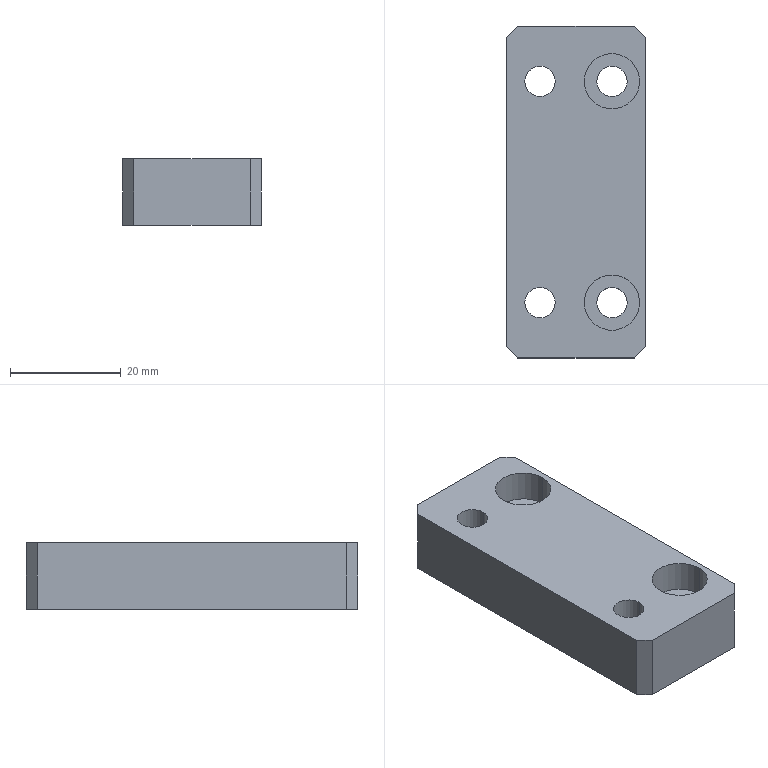Part | SolidWorks | features HoleWzd 2, Chamfer 1, Extrusion 1 | 1 solid | 30 faces | box 25 x 60 x 12 mm | volume 15515 mm3 | cylinder 16 | plane 14 | commonest cylinder face diameters 5.5 x8 10 x8
STEP:
#1=CARTESIAN_POINT('',(1.5,20.,0.3));
#2=VERTEX_POINT('',#1);
#3=CARTESIAN_POINT('',(11.5,20.,0.3));
#4=VERTEX_POINT('',#3);
#5=CARTESIAN_POINT('',(6.5,20.,0.3));
#6=DIRECTION('',(0.,0.,1.));
#7=DIRECTION('',(1.,0.,0.));
#8=AXIS2_PLACEMENT_3D('',#5,#6,#7);
#9=CIRCLE('',#8,5.);
#10=EDGE_CURVE('',#2,#4,#9,.T.);
#11=ORIENTED_EDGE('',*,*,#10,.F.);
#12=CARTESIAN_POINT('',(1.5,20.,6.));
#13=VERTEX_POINT('',#12);
#14=CARTESIAN_POINT('',(1.5,20.,6.));
#15=DIRECTION('',(0.,0.,1.));
#16=VECTOR('',#15,1000.);
#17=LINE('',#14,#16);
#18=EDGE_CURVE('',#2,#13,#17,.T.);
#19=ORIENTED_EDGE('',*,*,#18,.T.);
#20=CARTESIAN_POINT('',(11.5,20.,6.));
#21=VERTEX_POINT('',#20);
#22=CARTESIAN_POINT('',(6.5,20.,6.));
#23=DIRECTION('',(0.,0.,1.));
#24=DIRECTION('',(1.,0.,0.));
#25=AXIS2_PLACEMENT_3D('',#22,#23,#24);
#26=CIRCLE('',#25,5.);
#27=EDGE_CURVE('',#13,#21,#26,.T.);
#28=ORIENTED_EDGE('',*,*,#27,.T.);
#29=CARTESIAN_POINT('',(11.5,20.,6.));
#30=DIRECTION('',(0.,0.,1.));
#31=VECTOR('',#30,1000.);
#32=LINE('',#29,#31);
#33=EDGE_CURVE('',#4,#21,#32,.T.);
#34=ORIENTED_EDGE('',*,*,#33,.F.);
#35=EDGE_LOOP('',(#11,#19,#28,#34));
#36=FACE_OUTER_BOUND('',#35,.T.);
#37=CARTESIAN_POINT('',(6.5,20.,6.));
#38=DIRECTION('',(0.,0.,1.));
#39=DIRECTION('',(1.,0.,0.));
#40=AXIS2_PLACEMENT_3D('',#37,#38,#39);
#41=CYLINDRICAL_SURFACE('',#40,5.);
#42=ADVANCED_FACE('',(#36),#41,.F.);
#43=CARTESIAN_POINT('',(9.25,20.,-6.));
#44=VERTEX_POINT('',#43);
#45=CARTESIAN_POINT('',(3.75,20.,-6.));
#46=VERTEX_POINT('',#45);
#47=CARTESIAN_POINT('',(6.5,20.,-6.));
#48=DIRECTION('',(0.,0.,-1.));
#49=DIRECTION('',(-1.,0.,0.));
#50=AXIS2_PLACEMENT_3D('',#47,#48,#49);
#51=CIRCLE('',#50,2.75);
#52=EDGE_CURVE('',#44,#46,#51,.T.);
#53=ORIENTED_EDGE('',*,*,#52,.T.);
#54=CARTESIAN_POINT('',(3.75,20.,0.3));
#55=VERTEX_POINT('',#54);
#56=CARTESIAN_POINT('',(3.75,20.,6.));
#57=DIRECTION('',(0.,0.,1.));
#58=VECTOR('',#57,1000.);
#59=LINE('',#56,#58);
#60=EDGE_CURVE('',#46,#55,#59,.T.);
#61=ORIENTED_EDGE('',*,*,#60,.T.);
#62=CARTESIAN_POINT('',(9.25,20.,0.3));
#63=VERTEX_POINT('',#62);
#64=CARTESIAN_POINT('',(6.5,20.,0.3));
#65=DIRECTION('',(0.,0.,1.));
#66=DIRECTION('',(1.,0.,0.));
#67=AXIS2_PLACEMENT_3D('',#64,#65,#66);
#68=CIRCLE('',#67,2.75);
#69=EDGE_CURVE('',#55,#63,#68,.T.);
#70=ORIENTED_EDGE('',*,*,#69,.T.);
#71=CARTESIAN_POINT('',(9.25,20.,6.));
#72=DIRECTION('',(0.,0.,1.));
#73=VECTOR('',#72,1000.);
#74=LINE('',#71,#73);
#75=EDGE_CURVE('',#44,#63,#74,.T.);
#76=ORIENTED_EDGE('',*,*,#75,.F.);
#77=EDGE_LOOP('',(#53,#61,#70,#76));
#78=FACE_OUTER_BOUND('',#77,.T.);
#79=CARTESIAN_POINT('',(6.5,20.,6.));
#80=DIRECTION('',(0.,0.,1.));
#81=DIRECTION('',(1.,0.,0.));
#82=AXIS2_PLACEMENT_3D('',#79,#80,#81);
#83=CYLINDRICAL_SURFACE('',#82,2.75);
#84=ADVANCED_FACE('',(#78),#83,.F.);
#85=CARTESIAN_POINT('',(1.5,-20.,0.3));
#86=VERTEX_POINT('',#85);
#87=CARTESIAN_POINT('',(11.5,-20.,0.3));
#88=VERTEX_POINT('',#87);
#89=CARTESIAN_POINT('',(6.5,-20.,0.3));
#90=DIRECTION('',(0.,0.,1.));
#91=DIRECTION('',(1.,0.,0.));
#92=AXIS2_PLACEMENT_3D('',#89,#90,#91);
#93=CIRCLE('',#92,5.);
#94=EDGE_CURVE('',#86,#88,#93,.T.);
#95=ORIENTED_EDGE('',*,*,#94,.F.);
#96=CARTESIAN_POINT('',(1.5,-20.,6.));
#97=VERTEX_POINT('',#96);
#98=CARTESIAN_POINT('',(1.5,-20.,6.));
#99=DIRECTION('',(0.,0.,1.));
#100=VECTOR('',#99,1000.);
#101=LINE('',#98,#100);
#102=EDGE_CURVE('',#86,#97,#101,.T.);
#103=ORIENTED_EDGE('',*,*,#102,.T.);
#104=CARTESIAN_POINT('',(11.5,-20.,6.));
#105=VERTEX_POINT('',#104);
#106=CARTESIAN_POINT('',(6.5,-20.,6.));
#107=DIRECTION('',(0.,0.,1.));
#108=DIRECTION('',(1.,0.,0.));
#109=AXIS2_PLACEMENT_3D('',#106,#107,#108);
#110=CIRCLE('',#109,5.);
#111=EDGE_CURVE('',#97,#105,#110,.T.);
#112=ORIENTED_EDGE('',*,*,#111,.T.);
#113=CARTESIAN_POINT('',(11.5,-20.,6.));
#114=DIRECTION('',(0.,0.,1.));
#115=VECTOR('',#114,1000.);
#116=LINE('',#113,#115);
#117=EDGE_CURVE('',#88,#105,#116,.T.);
#118=ORIENTED_EDGE('',*,*,#117,.F.);
#119=EDGE_LOOP('',(#95,#103,#112,#118));
#120=FACE_OUTER_BOUND('',#119,.T.);
#121=CARTESIAN_POINT('',(6.5,-20.,6.));
#122=DIRECTION('',(0.,0.,1.));
#123=DIRECTION('',(1.,0.,0.));
#124=AXIS2_PLACEMENT_3D('',#121,#122,#123);
#125=CYLINDRICAL_SURFACE('',#124,5.);
#126=ADVANCED_FACE('',(#120),#125,.F.);
#127=CARTESIAN_POINT('',(9.25,-20.,-6.));
#128=VERTEX_POINT('',#127);
#129=CARTESIAN_POINT('',(3.75,-20.,-6.));
#130=VERTEX_POINT('',#129);
#131=CARTESIAN_POINT('',(6.5,-20.,-6.));
#132=DIRECTION('',(0.,0.,-1.));
#133=DIRECTION('',(-1.,0.,0.));
#134=AXIS2_PLACEMENT_3D('',#131,#132,#133);
#135=CIRCLE('',#134,2.75);
#136=EDGE_CURVE('',#128,#130,#135,.T.);
#137=ORIENTED_EDGE('',*,*,#136,.T.);
#138=CARTESIAN_POINT('',(3.75,-20.,0.3));
#139=VERTEX_POINT('',#138);
#140=CARTESIAN_POINT('',(3.75,-20.,6.));
#141=DIRECTION('',(0.,0.,1.));
#142=VECTOR('',#141,1000.);
#143=LINE('',#140,#142);
#144=EDGE_CURVE('',#130,#139,#143,.T.);
#145=ORIENTED_EDGE('',*,*,#144,.T.);
#146=CARTESIAN_POINT('',(9.25,-20.,0.3));
#147=VERTEX_POINT('',#146);
#148=CARTESIAN_POINT('',(6.5,-20.,0.3));
#149=DIRECTION('',(0.,0.,1.));
#150=DIRECTION('',(1.,0.,0.));
#151=AXIS2_PLACEMENT_3D('',#148,#149,#150);
#152=CIRCLE('',#151,2.75);
#153=EDGE_CURVE('',#139,#147,#152,.T.);
#154=ORIENTED_EDGE('',*,*,#153,.T.);
#155=CARTESIAN_POINT('',(9.25,-20.,6.));
#156=DIRECTION('',(0.,0.,1.));
#157=VECTOR('',#156,1000.);
#158=LINE('',#155,#157);
#159=EDGE_CURVE('',#128,#147,#158,.T.);
#160=ORIENTED_EDGE('',*,*,#159,.F.);
#161=EDGE_LOOP('',(#137,#145,#154,#160));
#162=FACE_OUTER_BOUND('',#161,.T.);
#163=CARTESIAN_POINT('',(6.5,-20.,6.));
#164=DIRECTION('',(0.,0.,1.));
#165=DIRECTION('',(1.,0.,0.));
#166=AXIS2_PLACEMENT_3D('',#163,#164,#165);
#167=CYLINDRICAL_SURFACE('',#166,2.75);
#168=ADVANCED_FACE('',(#162),#167,.F.);
#169=CARTESIAN_POINT('',(-1.5,20.,-0.3));
#170=VERTEX_POINT('',#169);
#171=CARTESIAN_POINT('',(-11.5,20.,-0.3));
#172=VERTEX_POINT('',#171);
#173=CARTESIAN_POINT('',(-6.5,20.,-0.3));
#174=DIRECTION('',(0.,0.,-1.));
#175=DIRECTION('',(-1.,0.,0.));
#176=AXIS2_PLACEMENT_3D('',#173,#174,#175);
#177=CIRCLE('',#176,5.);
#178=EDGE_CURVE('',#170,#172,#177,.T.);
#179=ORIENTED_EDGE('',*,*,#178,.F.);
#180=CARTESIAN_POINT('',(-1.5,20.,-6.));
#181=VERTEX_POINT('',#180);
#182=CARTESIAN_POINT('',(-1.5,20.,-6.));
#183=DIRECTION('',(0.,0.,-1.));
#184=VECTOR('',#183,1000.);
#185=LINE('',#182,#184);
#186=EDGE_CURVE('',#170,#181,#185,.T.);
#187=ORIENTED_EDGE('',*,*,#186,.T.);
#188=CARTESIAN_POINT('',(-11.5,20.,-6.));
#189=VERTEX_POINT('',#188);
#190=CARTESIAN_POINT('',(-6.5,20.,-6.));
#191=DIRECTION('',(0.,0.,-1.));
#192=DIRECTION('',(-1.,0.,0.));
#193=AXIS2_PLACEMENT_3D('',#190,#191,#192);
#194=CIRCLE('',#193,5.);
#195=EDGE_CURVE('',#181,#189,#194,.T.);
#196=ORIENTED_EDGE('',*,*,#195,.T.);
#197=CARTESIAN_POINT('',(-11.5,20.,-6.));
#198=DIRECTION('',(0.,0.,-1.));
#199=VECTOR('',#198,1000.);
#200=LINE('',#197,#199);
#201=EDGE_CURVE('',#172,#189,#200,.T.);
#202=ORIENTED_EDGE('',*,*,#201,.F.);
#203=EDGE_LOOP('',(#179,#187,#196,#202));
#204=FACE_OUTER_BOUND('',#203,.T.);
#205=CARTESIAN_POINT('',(-6.5,20.,-6.));
#206=DIRECTION('',(0.,0.,-1.));
#207=DIRECTION('',(-1.,0.,0.));
#208=AXIS2_PLACEMENT_3D('',#205,#206,#207);
#209=CYLINDRICAL_SURFACE('',#208,5.);
#210=ADVANCED_FACE('',(#204),#209,.F.);
#211=CARTESIAN_POINT('',(-3.75,20.,6.));
#212=VERTEX_POINT('',#211);
#213=CARTESIAN_POINT('',(-9.25,20.,6.));
#214=VERTEX_POINT('',#213);
#215=CARTESIAN_POINT('',(-6.5,20.,6.));
#216=DIRECTION('',(0.,0.,-1.));
#217=DIRECTION('',(-1.,0.,0.));
#218=AXIS2_PLACEMENT_3D('',#215,#216,#217);
#219=CIRCLE('',#218,2.75);
#220=EDGE_CURVE('',#212,#214,#219,.T.);
#221=ORIENTED_EDGE('',*,*,#220,.F.);
#222=CARTESIAN_POINT('',(-3.75,20.,-0.3));
#223=VERTEX_POINT('',#222);
#224=CARTESIAN_POINT('',(-3.75,20.,-6.));
#225=DIRECTION('',(0.,0.,-1.));
#226=VECTOR('',#225,1000.);
#227=LINE('',#224,#226);
#228=EDGE_CURVE('',#212,#223,#227,.T.);
#229=ORIENTED_EDGE('',*,*,#228,.T.);
#230=CARTESIAN_POINT('',(-9.25,20.,-0.3));
#231=VERTEX_POINT('',#230);
#232=CARTESIAN_POINT('',(-6.5,20.,-0.3));
#233=DIRECTION('',(0.,0.,-1.));
#234=DIRECTION('',(-1.,0.,0.));
#235=AXIS2_PLACEMENT_3D('',#232,#233,#234);
#236=CIRCLE('',#235,2.75);
#237=EDGE_CURVE('',#223,#231,#236,.T.);
#238=ORIENTED_EDGE('',*,*,#237,.T.);
#239=CARTESIAN_POINT('',(-9.25,20.,-6.));
#240=DIRECTION('',(0.,0.,-1.));
#241=VECTOR('',#240,1000.);
#242=LINE('',#239,#241);
#243=EDGE_CURVE('',#214,#231,#242,.T.);
#244=ORIENTED_EDGE('',*,*,#243,.F.);
#245=EDGE_LOOP('',(#221,#229,#238,#244));
#246=FACE_OUTER_BOUND('',#245,.T.);
#247=CARTESIAN_POINT('',(-6.5,20.,-6.));
#248=DIRECTION('',(0.,0.,-1.));
#249=DIRECTION('',(-1.,0.,0.));
#250=AXIS2_PLACEMENT_3D('',#247,#248,#249);
#251=CYLINDRICAL_SURFACE('',#250,2.75);
#252=ADVANCED_FACE('',(#246),#251,.F.);
#253=CARTESIAN_POINT('',(-1.5,-20.,-0.3));
#254=VERTEX_POINT('',#253);
#255=CARTESIAN_POINT('',(-11.5,-20.,-0.3));
#256=VERTEX_POINT('',#255);
#257=CARTESIAN_POINT('',(-6.5,-20.,-0.3));
#258=DIRECTION('',(0.,0.,-1.));
#259=DIRECTION('',(-1.,0.,0.));
#260=AXIS2_PLACEMENT_3D('',#257,#258,#259);
#261=CIRCLE('',#260,5.);
#262=EDGE_CURVE('',#254,#256,#261,.T.);
#263=ORIENTED_EDGE('',*,*,#262,.F.);
#264=CARTESIAN_POINT('',(-1.5,-20.,-6.));
#265=VERTEX_POINT('',#264);
#266=CARTESIAN_POINT('',(-1.5,-20.,-6.));
#267=DIRECTION('',(0.,0.,-1.));
#268=VECTOR('',#267,1000.);
#269=LINE('',#266,#268);
#270=EDGE_CURVE('',#254,#265,#269,.T.);
#271=ORIENTED_EDGE('',*,*,#270,.T.);
#272=CARTESIAN_POINT('',(-11.5,-20.,-6.));
#273=VERTEX_POINT('',#272);
#274=CARTESIAN_POINT('',(-6.5,-20.,-6.));
#275=DIRECTION('',(0.,0.,-1.));
#276=DIRECTION('',(-1.,0.,0.));
#277=AXIS2_PLACEMENT_3D('',#274,#275,#276);
#278=CIRCLE('',#277,5.);
#279=EDGE_CURVE('',#265,#273,#278,.T.);
#280=ORIENTED_EDGE('',*,*,#279,.T.);
#281=CARTESIAN_POINT('',(-11.5,-20.,-6.));
#282=DIRECTION('',(0.,0.,-1.));
#283=VECTOR('',#282,1000.);
#284=LINE('',#281,#283);
#285=EDGE_CURVE('',#256,#273,#284,.T.);
#286=ORIENTED_EDGE('',*,*,#285,.F.);
#287=EDGE_LOOP('',(#263,#271,#280,#286));
#288=FACE_OUTER_BOUND('',#287,.T.);
#289=CARTESIAN_POINT('',(-6.5,-20.,-6.));
#290=DIRECTION('',(0.,0.,-1.));
#291=DIRECTION('',(-1.,0.,0.));
#292=AXIS2_PLACEMENT_3D('',#289,#290,#291);
#293=CYLINDRICAL_SURFACE('',#292,5.);
#294=ADVANCED_FACE('',(#288),#293,.F.);
#295=CARTESIAN_POINT('',(-3.75,-20.,6.));
#296=VERTEX_POINT('',#295);
#297=CARTESIAN_POINT('',(-9.25,-20.,6.));
#298=VERTEX_POINT('',#297);
#299=CARTESIAN_POINT('',(-6.5,-20.,6.));
#300=DIRECTION('',(0.,0.,-1.));
#301=DIRECTION('',(-1.,0.,0.));
#302=AXIS2_PLACEMENT_3D('',#299,#300,#301);
#303=CIRCLE('',#302,2.75);
#304=EDGE_CURVE('',#296,#298,#303,.T.);
#305=ORIENTED_EDGE('',*,*,#304,.F.);
#306=CARTESIAN_POINT('',(-3.75,-20.,-0.3));
#307=VERTEX_POINT('',#306);
#308=CARTESIAN_POINT('',(-3.75,-20.,-6.));
#309=DIRECTION('',(0.,0.,-1.));
#310=VECTOR('',#309,1000.);
#311=LINE('',#308,#310);
#312=EDGE_CURVE('',#296,#307,#311,.T.);
#313=ORIENTED_EDGE('',*,*,#312,.T.);
#314=CARTESIAN_POINT('',(-9.25,-20.,-0.3));
#315=VERTEX_POINT('',#314);
#316=CARTESIAN_POINT('',(-6.5,-20.,-0.3));
#317=DIRECTION('',(0.,0.,-1.));
#318=DIRECTION('',(-1.,0.,0.));
#319=AXIS2_PLACEMENT_3D('',#316,#317,#318);
#320=CIRCLE('',#319,2.75);
#321=EDGE_CURVE('',#307,#315,#320,.T.);
#322=ORIENTED_EDGE('',*,*,#321,.T.);
#323=CARTESIAN_POINT('',(-9.25,-20.,-6.));
#324=DIRECTION('',(0.,0.,-1.));
#325=VECTOR('',#324,1000.);
#326=LINE('',#323,#325);
#327=EDGE_CURVE('',#298,#315,#326,.T.);
#328=ORIENTED_EDGE('',*,*,#327,.F.);
#329=EDGE_LOOP('',(#305,#313,#322,#328));
#330=FACE_OUTER_BOUND('',#329,.T.);
#331=CARTESIAN_POINT('',(-6.5,-20.,-6.));
#332=DIRECTION('',(0.,0.,-1.));
#333=DIRECTION('',(-1.,0.,0.));
#334=AXIS2_PLACEMENT_3D('',#331,#332,#333);
#335=CYLINDRICAL_SURFACE('',#334,2.75);
#336=ADVANCED_FACE('',(#330),#335,.F.);
#337=CARTESIAN_POINT('',(12.5,-28.,6.));
#338=VERTEX_POINT('',#337);
#339=CARTESIAN_POINT('',(12.5,28.,6.));
#340=VERTEX_POINT('',#339);
#341=CARTESIAN_POINT('',(12.5,-30.,6.));
#342=DIRECTION('',(0.,1.,0.));
#343=VECTOR('',#342,1000.);
#344=LINE('',#341,#343);
#345=EDGE_CURVE('',#338,#340,#344,.T.);
#346=ORIENTED_EDGE('',*,*,#345,.F.);
#347=CARTESIAN_POINT('',(12.5,-28.,-6.));
#348=VERTEX_POINT('',#347);
#349=CARTESIAN_POINT('',(12.5,-28.,6.));
#350=DIRECTION('',(0.,0.,-1.));
#351=VECTOR('',#350,1000.);
#352=LINE('',#349,#351);
#353=EDGE_CURVE('',#338,#348,#352,.T.);
#354=ORIENTED_EDGE('',*,*,#353,.T.);
#355=CARTESIAN_POINT('',(12.5,28.,-6.));
#356=VERTEX_POINT('',#355);
#357=CARTESIAN_POINT('',(12.5,-30.,-6.));
#358=DIRECTION('',(0.,1.,0.));
#359=VECTOR('',#358,1000.);
#360=LINE('',#357,#359);
#361=EDGE_CURVE('',#348,#356,#360,.T.);
#362=ORIENTED_EDGE('',*,*,#361,.T.);
#363=CARTESIAN_POINT('',(12.5,28.,6.));
#364=DIRECTION('',(0.,0.,1.));
#365=VECTOR('',#364,1000.);
#366=LINE('',#363,#365);
#367=EDGE_CURVE('',#356,#340,#366,.T.);
#368=ORIENTED_EDGE('',*,*,#367,.T.);
#369=EDGE_LOOP('',(#346,#354,#362,#368));
#370=FACE_OUTER_BOUND('',#369,.T.);
#371=CARTESIAN_POINT('',(12.5,-30.,6.));
#372=DIRECTION('',(-1.,0.,0.));
#373=DIRECTION('',(0.,0.,1.));
#374=AXIS2_PLACEMENT_3D('',#371,#372,#373);
#375=PLANE('',#374);
#376=ADVANCED_FACE('',(#370),#375,.F.);
#377=CARTESIAN_POINT('',(10.5,30.,-6.));
#378=VERTEX_POINT('',#377);
#379=CARTESIAN_POINT('',(-10.5,30.,-6.));
#380=VERTEX_POINT('',#379);
#381=CARTESIAN_POINT('',(-12.5,30.,-6.));
#382=DIRECTION('',(-1.,0.,0.));
#383=VECTOR('',#382,1000.);
#384=LINE('',#381,#383);
#385=EDGE_CURVE('',#378,#380,#384,.T.);
#386=ORIENTED_EDGE('',*,*,#385,.T.);
#387=CARTESIAN_POINT('',(-10.5,30.,6.));
#388=VERTEX_POINT('',#387);
#389=CARTESIAN_POINT('',(-10.5,30.,6.));
#390=DIRECTION('',(0.,0.,1.));
#391=VECTOR('',#390,1000.);
#392=LINE('',#389,#391);
#393=EDGE_CURVE('',#380,#388,#392,.T.);
#394=ORIENTED_EDGE('',*,*,#393,.T.);
#395=CARTESIAN_POINT('',(10.5,30.,6.));
#396=VERTEX_POINT('',#395);
#397=CARTESIAN_POINT('',(-12.5,30.,6.));
#398=DIRECTION('',(-1.,0.,0.));
#399=VECTOR('',#398,1000.);
#400=LINE('',#397,#399);
#401=EDGE_CURVE('',#396,#388,#400,.T.);
#402=ORIENTED_EDGE('',*,*,#401,.F.);
#403=CARTESIAN_POINT('',(10.5,30.,6.));
#404=DIRECTION('',(0.,0.,-1.));
#405=VECTOR('',#404,1000.);
#406=LINE('',#403,#405);
#407=EDGE_CURVE('',#396,#378,#406,.T.);
#408=ORIENTED_EDGE('',*,*,#407,.T.);
#409=EDGE_LOOP('',(#386,#394,#402,#408));
#410=FACE_OUTER_BOUND('',#409,.T.);
#411=CARTESIAN_POINT('',(-12.5,30.,6.));
#412=DIRECTION('',(0.,-1.,0.));
#413=DIRECTION('',(0.,0.,-1.));
#414=AXIS2_PLACEMENT_3D('',#411,#412,#413);
#415=PLANE('',#414);
#416=ADVANCED_FACE('',(#410),#415,.F.);
#417=CARTESIAN_POINT('',(-12.5,28.,-6.));
#418=VERTEX_POINT('',#417);
#419=CARTESIAN_POINT('',(-12.5,-28.,-6.));
#420=VERTEX_POINT('',#419);
#421=CARTESIAN_POINT('',(-12.5,-30.,-6.));
#422=DIRECTION('',(0.,-1.,0.));
#423=VECTOR('',#422,1000.);
#424=LINE('',#421,#423);
#425=EDGE_CURVE('',#418,#420,#424,.T.);
#426=ORIENTED_EDGE('',*,*,#425,.T.);
#427=CARTESIAN_POINT('',(-12.5,-28.,6.));
#428=VERTEX_POINT('',#427);
#429=CARTESIAN_POINT('',(-12.5,-28.,6.));
#430=DIRECTION('',(0.,0.,1.));
#431=VECTOR('',#430,1000.);
#432=LINE('',#429,#431);
#433=EDGE_CURVE('',#420,#428,#432,.T.);
#434=ORIENTED_EDGE('',*,*,#433,.T.);
#435=CARTESIAN_POINT('',(-12.5,28.,6.));
#436=VERTEX_POINT('',#435);
#437=CARTESIAN_POINT('',(-12.5,-30.,6.));
#438=DIRECTION('',(0.,-1.,0.));
#439=VECTOR('',#438,1000.);
#440=LINE('',#437,#439);
#441=EDGE_CURVE('',#436,#428,#440,.T.);
#442=ORIENTED_EDGE('',*,*,#441,.F.);
#443=CARTESIAN_POINT('',(-12.5,28.,6.));
#444=DIRECTION('',(0.,0.,-1.));
#445=VECTOR('',#444,1000.);
#446=LINE('',#443,#445);
#447=EDGE_CURVE('',#436,#418,#446,.T.);
#448=ORIENTED_EDGE('',*,*,#447,.T.);
#449=EDGE_LOOP('',(#426,#434,#442,#448));
#450=FACE_OUTER_BOUND('',#449,.T.);
#451=CARTESIAN_POINT('',(-12.5,-30.,6.));
#452=DIRECTION('',(1.,0.,0.));
#453=DIRECTION('',(0.,0.,-1.));
#454=AXIS2_PLACEMENT_3D('',#451,#452,#453);
#455=PLANE('',#454);
#456=ADVANCED_FACE('',(#450),#455,.F.);
#457=CARTESIAN_POINT('',(-10.5,-30.,-6.));
#458=VERTEX_POINT('',#457);
#459=CARTESIAN_POINT('',(10.5,-30.,-6.));
#460=VERTEX_POINT('',#459);
#461=CARTESIAN_POINT('',(-12.5,-30.,-6.));
#462=DIRECTION('',(1.,0.,0.));
#463=VECTOR('',#462,1000.);
#464=LINE('',#461,#463);
#465=EDGE_CURVE('',#458,#460,#464,.T.);
#466=ORIENTED_EDGE('',*,*,#465,.T.);
#467=CARTESIAN_POINT('',(10.5,-30.,6.));
#468=VERTEX_POINT('',#467);
#469=CARTESIAN_POINT('',(10.5,-30.,6.));
#470=DIRECTION('',(0.,0.,1.));
#471=VECTOR('',#470,1000.);
#472=LINE('',#469,#471);
#473=EDGE_CURVE('',#460,#468,#472,.T.);
#474=ORIENTED_EDGE('',*,*,#473,.T.);
#475=CARTESIAN_POINT('',(-10.5,-30.,6.));
#476=VERTEX_POINT('',#475);
#477=CARTESIAN_POINT('',(-12.5,-30.,6.));
#478=DIRECTION('',(1.,0.,0.));
#479=VECTOR('',#478,1000.);
#480=LINE('',#477,#479);
#481=EDGE_CURVE('',#476,#468,#480,.T.);
#482=ORIENTED_EDGE('',*,*,#481,.F.);
#483=CARTESIAN_POINT('',(-10.5,-30.,6.));
#484=DIRECTION('',(0.,0.,-1.));
#485=VECTOR('',#484,1000.);
#486=LINE('',#483,#485);
#487=EDGE_CURVE('',#476,#458,#486,.T.);
#488=ORIENTED_EDGE('',*,*,#487,.T.);
#489=EDGE_LOOP('',(#466,#474,#482,#488));
#490=FACE_OUTER_BOUND('',#489,.T.);
#491=CARTESIAN_POINT('',(-12.5,-30.,6.));
#492=DIRECTION('',(0.,1.,0.));
#493=DIRECTION('',(0.,0.,1.));
#494=AXIS2_PLACEMENT_3D('',#491,#492,#493);
#495=PLANE('',#494);
#496=ADVANCED_FACE('',(#490),#495,.F.);
#497=CARTESIAN_POINT('',(6.5,20.,6.));
#498=DIRECTION('',(0.,0.,1.));
#499=DIRECTION('',(1.,0.,0.));
#500=AXIS2_PLACEMENT_3D('',#497,#498,#499);
#501=CIRCLE('',#500,5.);
#502=EDGE_CURVE('',#21,#13,#501,.T.);
#503=ORIENTED_EDGE('',*,*,#502,.F.);
#504=ORIENTED_EDGE('',*,*,#27,.F.);
#505=EDGE_LOOP('',(#503,#504));
#506=FACE_BOUND('',#505,.T.);
#507=CARTESIAN_POINT('',(6.5,-20.,6.));
#508=DIRECTION('',(0.,0.,1.));
#509=DIRECTION('',(1.,0.,0.));
#510=AXIS2_PLACEMENT_3D('',#507,#508,#509);
#511=CIRCLE('',#510,5.);
#512=EDGE_CURVE('',#105,#97,#511,.T.);
#513=ORIENTED_EDGE('',*,*,#512,.F.);
#514=ORIENTED_EDGE('',*,*,#111,.F.);
#515=EDGE_LOOP('',(#513,#514));
#516=FACE_BOUND('',#515,.T.);
#517=CARTESIAN_POINT('',(-6.5,20.,6.));
#518=DIRECTION('',(0.,0.,-1.));
#519=DIRECTION('',(-1.,0.,0.));
#520=AXIS2_PLACEMENT_3D('',#517,#518,#519);
#521=CIRCLE('',#520,2.75);
#522=EDGE_CURVE('',#214,#212,#521,.T.);
#523=ORIENTED_EDGE('',*,*,#522,.T.);
#524=ORIENTED_EDGE('',*,*,#220,.T.);
#525=EDGE_LOOP('',(#523,#524));
#526=FACE_BOUND('',#525,.T.);
#527=CARTESIAN_POINT('',(-6.5,-20.,6.));
#528=DIRECTION('',(0.,0.,-1.));
#529=DIRECTION('',(-1.,0.,0.));
#530=AXIS2_PLACEMENT_3D('',#527,#528,#529);
#531=CIRCLE('',#530,2.75);
#532=EDGE_CURVE('',#298,#296,#531,.T.);
#533=ORIENTED_EDGE('',*,*,#532,.T.);
#534=ORIENTED_EDGE('',*,*,#304,.T.);
#535=EDGE_LOOP('',(#533,#534));
#536=FACE_BOUND('',#535,.T.);
#537=ORIENTED_EDGE('',*,*,#481,.T.);
#538=CARTESIAN_POINT('',(12.5,-28.,6.));
#539=DIRECTION('',(0.7071,0.7071,0.));
#540=VECTOR('',#539,1000.);
#541=LINE('',#538,#540);
#542=EDGE_CURVE('',#468,#338,#541,.T.);
#543=ORIENTED_EDGE('',*,*,#542,.T.);
#544=ORIENTED_EDGE('',*,*,#345,.T.);
#545=CARTESIAN_POINT('',(10.5,30.,6.));
#546=DIRECTION('',(-0.7071,0.7071,0.));
#547=VECTOR('',#546,1000.);
#548=LINE('',#545,#547);
#549=EDGE_CURVE('',#340,#396,#548,.T.);
#550=ORIENTED_EDGE('',*,*,#549,.T.);
#551=ORIENTED_EDGE('',*,*,#401,.T.);
#552=CARTESIAN_POINT('',(-12.5,28.,6.));
#553=DIRECTION('',(-0.7071,-0.7071,0.));
#554=VECTOR('',#553,1000.);
#555=LINE('',#552,#554);
#556=EDGE_CURVE('',#388,#436,#555,.T.);
#557=ORIENTED_EDGE('',*,*,#556,.T.);
#558=ORIENTED_EDGE('',*,*,#441,.T.);
#559=CARTESIAN_POINT('',(-10.5,-30.,6.));
#560=DIRECTION('',(0.7071,-0.7071,0.));
#561=VECTOR('',#560,1000.);
#562=LINE('',#559,#561);
#563=EDGE_CURVE('',#428,#476,#562,.T.);
#564=ORIENTED_EDGE('',*,*,#563,.T.);
#565=EDGE_LOOP('',(#537,#543,#544,#550,#551,#557,#558,#564));
#566=FACE_OUTER_BOUND('',#565,.T.);
#567=CARTESIAN_POINT('',(0.,0.,6.));
#568=DIRECTION('',(0.,0.,-1.));
#569=DIRECTION('',(-1.,0.,0.));
#570=AXIS2_PLACEMENT_3D('',#567,#568,#569);
#571=PLANE('',#570);
#572=ADVANCED_FACE('',(#506,#516,#526,#536,#566),#571,.F.);
#573=ORIENTED_EDGE('',*,*,#52,.F.);
#574=CARTESIAN_POINT('',(6.5,20.,-6.));
#575=DIRECTION('',(0.,0.,-1.));
#576=DIRECTION('',(-1.,0.,0.));
#577=AXIS2_PLACEMENT_3D('',#574,#575,#576);
#578=CIRCLE('',#577,2.75);
#579=EDGE_CURVE('',#46,#44,#578,.T.);
#580=ORIENTED_EDGE('',*,*,#579,.F.);
#581=EDGE_LOOP('',(#573,#580));
#582=FACE_BOUND('',#581,.T.);
#583=ORIENTED_EDGE('',*,*,#136,.F.);
#584=CARTESIAN_POINT('',(6.5,-20.,-6.));
#585=DIRECTION('',(0.,0.,-1.));
#586=DIRECTION('',(-1.,0.,0.));
#587=AXIS2_PLACEMENT_3D('',#584,#585,#586);
#588=CIRCLE('',#587,2.75);
#589=EDGE_CURVE('',#130,#128,#588,.T.);
#590=ORIENTED_EDGE('',*,*,#589,.F.);
#591=EDGE_LOOP('',(#583,#590));
#592=FACE_BOUND('',#591,.T.);
#593=CARTESIAN_POINT('',(-6.5,20.,-6.));
#594=DIRECTION('',(0.,0.,-1.));
#595=DIRECTION('',(-1.,0.,0.));
#596=AXIS2_PLACEMENT_3D('',#593,#594,#595);
#597=CIRCLE('',#596,5.);
#598=EDGE_CURVE('',#189,#181,#597,.T.);
#599=ORIENTED_EDGE('',*,*,#598,.F.);
#600=ORIENTED_EDGE('',*,*,#195,.F.);
#601=EDGE_LOOP('',(#599,#600));
#602=FACE_BOUND('',#601,.T.);
#603=CARTESIAN_POINT('',(-6.5,-20.,-6.));
#604=DIRECTION('',(0.,0.,-1.));
#605=DIRECTION('',(-1.,0.,0.));
#606=AXIS2_PLACEMENT_3D('',#603,#604,#605);
#607=CIRCLE('',#606,5.);
#608=EDGE_CURVE('',#273,#265,#607,.T.);
#609=ORIENTED_EDGE('',*,*,#608,.F.);
#610=ORIENTED_EDGE('',*,*,#279,.F.);
#611=EDGE_LOOP('',(#609,#610));
#612=FACE_BOUND('',#611,.T.);
#613=ORIENTED_EDGE('',*,*,#361,.F.);
#614=CARTESIAN_POINT('',(20.25,-20.25,-6.));
#615=DIRECTION('',(-0.7071,-0.7071,0.));
#616=VECTOR('',#615,1000.);
#617=LINE('',#614,#616);
#618=EDGE_CURVE('',#348,#460,#617,.T.);
#619=ORIENTED_EDGE('',*,*,#618,.T.);
#620=ORIENTED_EDGE('',*,*,#465,.F.);
#621=CARTESIAN_POINT('',(-20.25,-20.25,-6.));
#622=DIRECTION('',(-0.7071,0.7071,0.));
#623=VECTOR('',#622,1000.);
#624=LINE('',#621,#623);
#625=EDGE_CURVE('',#458,#420,#624,.T.);
#626=ORIENTED_EDGE('',*,*,#625,.T.);
#627=ORIENTED_EDGE('',*,*,#425,.F.);
#628=CARTESIAN_POINT('',(-20.25,20.25,-6.));
#629=DIRECTION('',(0.7071,0.7071,0.));
#630=VECTOR('',#629,1000.);
#631=LINE('',#628,#630);
#632=EDGE_CURVE('',#418,#380,#631,.T.);
#633=ORIENTED_EDGE('',*,*,#632,.T.);
#634=ORIENTED_EDGE('',*,*,#385,.F.);
#635=CARTESIAN_POINT('',(20.25,20.25,-6.));
#636=DIRECTION('',(0.7071,-0.7071,0.));
#637=VECTOR('',#636,1000.);
#638=LINE('',#635,#637);
#639=EDGE_CURVE('',#378,#356,#638,.T.);
#640=ORIENTED_EDGE('',*,*,#639,.T.);
#641=EDGE_LOOP('',(#613,#619,#620,#626,#627,#633,#634,#640));
#642=FACE_OUTER_BOUND('',#641,.T.);
#643=CARTESIAN_POINT('',(0.,0.,-6.));
#644=DIRECTION('',(0.,0.,-1.));
#645=DIRECTION('',(-1.,0.,0.));
#646=AXIS2_PLACEMENT_3D('',#643,#644,#645);
#647=PLANE('',#646);
#648=ADVANCED_FACE('',(#582,#592,#602,#612,#642),#647,.T.);
#649=ORIENTED_EDGE('',*,*,#542,.F.);
#650=ORIENTED_EDGE('',*,*,#473,.F.);
#651=ORIENTED_EDGE('',*,*,#618,.F.);
#652=ORIENTED_EDGE('',*,*,#353,.F.);
#653=EDGE_LOOP('',(#649,#650,#651,#652));
#654=FACE_OUTER_BOUND('',#653,.T.);
#655=CARTESIAN_POINT('',(12.5,-28.,6.));
#656=DIRECTION('',(-0.7071,0.7071,0.));
#657=DIRECTION('',(0.,0.,-1.));
#658=AXIS2_PLACEMENT_3D('',#655,#656,#657);
#659=PLANE('',#658);
#660=ADVANCED_FACE('',(#654),#659,.F.);
#661=ORIENTED_EDGE('',*,*,#563,.F.);
#662=ORIENTED_EDGE('',*,*,#433,.F.);
#663=ORIENTED_EDGE('',*,*,#625,.F.);
#664=ORIENTED_EDGE('',*,*,#487,.F.);
#665=EDGE_LOOP('',(#661,#662,#663,#664));
#666=FACE_OUTER_BOUND('',#665,.T.);
#667=CARTESIAN_POINT('',(-10.5,-30.,6.));
#668=DIRECTION('',(0.7071,0.7071,0.));
#669=DIRECTION('',(0.,0.,-1.));
#670=AXIS2_PLACEMENT_3D('',#667,#668,#669);
#671=PLANE('',#670);
#672=ADVANCED_FACE('',(#666),#671,.F.);
#673=ORIENTED_EDGE('',*,*,#556,.F.);
#674=ORIENTED_EDGE('',*,*,#393,.F.);
#675=ORIENTED_EDGE('',*,*,#632,.F.);
#676=ORIENTED_EDGE('',*,*,#447,.F.);
#677=EDGE_LOOP('',(#673,#674,#675,#676));
#678=FACE_OUTER_BOUND('',#677,.T.);
#679=CARTESIAN_POINT('',(-12.5,28.,6.));
#680=DIRECTION('',(0.7071,-0.7071,0.));
#681=DIRECTION('',(0.,0.,-1.));
#682=AXIS2_PLACEMENT_3D('',#679,#680,#681);
#683=PLANE('',#682);
#684=ADVANCED_FACE('',(#678),#683,.F.);
#685=ORIENTED_EDGE('',*,*,#549,.F.);
#686=ORIENTED_EDGE('',*,*,#367,.F.);
#687=ORIENTED_EDGE('',*,*,#639,.F.);
#688=ORIENTED_EDGE('',*,*,#407,.F.);
#689=EDGE_LOOP('',(#685,#686,#687,#688));
#690=FACE_OUTER_BOUND('',#689,.T.);
#691=CARTESIAN_POINT('',(10.5,30.,6.));
#692=DIRECTION('',(-0.7071,-0.7071,0.));
#693=DIRECTION('',(0.,0.,-1.));
#694=AXIS2_PLACEMENT_3D('',#691,#692,#693);
#695=PLANE('',#694);
#696=ADVANCED_FACE('',(#690),#695,.F.);
#697=ORIENTED_EDGE('',*,*,#312,.F.);
#698=ORIENTED_EDGE('',*,*,#532,.F.);
#699=ORIENTED_EDGE('',*,*,#327,.T.);
#700=CARTESIAN_POINT('',(-6.5,-20.,-0.3));
#701=DIRECTION('',(0.,0.,-1.));
#702=DIRECTION('',(-1.,0.,0.));
#703=AXIS2_PLACEMENT_3D('',#700,#701,#702);
#704=CIRCLE('',#703,2.75);
#705=EDGE_CURVE('',#315,#307,#704,.T.);
#706=ORIENTED_EDGE('',*,*,#705,.T.);
#707=EDGE_LOOP('',(#697,#698,#699,#706));
#708=FACE_OUTER_BOUND('',#707,.T.);
#709=CARTESIAN_POINT('',(-6.5,-20.,-6.));
#710=DIRECTION('',(0.,0.,-1.));
#711=DIRECTION('',(-1.,0.,0.));
#712=AXIS2_PLACEMENT_3D('',#709,#710,#711);
#713=CYLINDRICAL_SURFACE('',#712,2.75);
#714=ADVANCED_FACE('',(#708),#713,.F.);
#715=ORIENTED_EDGE('',*,*,#705,.F.);
#716=ORIENTED_EDGE('',*,*,#321,.F.);
#717=EDGE_LOOP('',(#715,#716));
#718=FACE_BOUND('',#717,.T.);
#719=CARTESIAN_POINT('',(-6.5,-20.,-0.3));
#720=DIRECTION('',(0.,0.,-1.));
#721=DIRECTION('',(-1.,0.,0.));
#722=AXIS2_PLACEMENT_3D('',#719,#720,#721);
#723=CIRCLE('',#722,5.);
#724=EDGE_CURVE('',#256,#254,#723,.T.);
#725=ORIENTED_EDGE('',*,*,#724,.T.);
#726=ORIENTED_EDGE('',*,*,#262,.T.);
#727=EDGE_LOOP('',(#725,#726));
#728=FACE_OUTER_BOUND('',#727,.T.);
#729=CARTESIAN_POINT('',(-3.75,-20.,-0.3));
#730=DIRECTION('',(0.,0.,1.));
#731=DIRECTION('',(1.,0.,0.));
#732=AXIS2_PLACEMENT_3D('',#729,#730,#731);
#733=PLANE('',#732);
#734=ADVANCED_FACE('',(#718,#728),#733,.F.);
#735=ORIENTED_EDGE('',*,*,#270,.F.);
#736=ORIENTED_EDGE('',*,*,#724,.F.);
#737=ORIENTED_EDGE('',*,*,#285,.T.);
#738=ORIENTED_EDGE('',*,*,#608,.T.);
#739=EDGE_LOOP('',(#735,#736,#737,#738));
#740=FACE_OUTER_BOUND('',#739,.T.);
#741=CARTESIAN_POINT('',(-6.5,-20.,-6.));
#742=DIRECTION('',(0.,0.,-1.));
#743=DIRECTION('',(-1.,0.,0.));
#744=AXIS2_PLACEMENT_3D('',#741,#742,#743);
#745=CYLINDRICAL_SURFACE('',#744,5.);
#746=ADVANCED_FACE('',(#740),#745,.F.);
#747=ORIENTED_EDGE('',*,*,#228,.F.);
#748=ORIENTED_EDGE('',*,*,#522,.F.);
#749=ORIENTED_EDGE('',*,*,#243,.T.);
#750=CARTESIAN_POINT('',(-6.5,20.,-0.3));
#751=DIRECTION('',(0.,0.,-1.));
#752=DIRECTION('',(-1.,0.,0.));
#753=AXIS2_PLACEMENT_3D('',#750,#751,#752);
#754=CIRCLE('',#753,2.75);
#755=EDGE_CURVE('',#231,#223,#754,.T.);
#756=ORIENTED_EDGE('',*,*,#755,.T.);
#757=EDGE_LOOP('',(#747,#748,#749,#756));
#758=FACE_OUTER_BOUND('',#757,.T.);
#759=CARTESIAN_POINT('',(-6.5,20.,-6.));
#760=DIRECTION('',(0.,0.,-1.));
#761=DIRECTION('',(-1.,0.,0.));
#762=AXIS2_PLACEMENT_3D('',#759,#760,#761);
#763=CYLINDRICAL_SURFACE('',#762,2.75);
#764=ADVANCED_FACE('',(#758),#763,.F.);
#765=ORIENTED_EDGE('',*,*,#755,.F.);
#766=ORIENTED_EDGE('',*,*,#237,.F.);
#767=EDGE_LOOP('',(#765,#766));
#768=FACE_BOUND('',#767,.T.);
#769=CARTESIAN_POINT('',(-6.5,20.,-0.3));
#770=DIRECTION('',(0.,0.,-1.));
#771=DIRECTION('',(-1.,0.,0.));
#772=AXIS2_PLACEMENT_3D('',#769,#770,#771);
#773=CIRCLE('',#772,5.);
#774=EDGE_CURVE('',#172,#170,#773,.T.);
#775=ORIENTED_EDGE('',*,*,#774,.T.);
#776=ORIENTED_EDGE('',*,*,#178,.T.);
#777=EDGE_LOOP('',(#775,#776));
#778=FACE_OUTER_BOUND('',#777,.T.);
#779=CARTESIAN_POINT('',(-3.75,20.,-0.3));
#780=DIRECTION('',(0.,0.,1.));
#781=DIRECTION('',(1.,0.,0.));
#782=AXIS2_PLACEMENT_3D('',#779,#780,#781);
#783=PLANE('',#782);
#784=ADVANCED_FACE('',(#768,#778),#783,.F.);
#785=ORIENTED_EDGE('',*,*,#186,.F.);
#786=ORIENTED_EDGE('',*,*,#774,.F.);
#787=ORIENTED_EDGE('',*,*,#201,.T.);
#788=ORIENTED_EDGE('',*,*,#598,.T.);
#789=EDGE_LOOP('',(#785,#786,#787,#788));
#790=FACE_OUTER_BOUND('',#789,.T.);
#791=CARTESIAN_POINT('',(-6.5,20.,-6.));
#792=DIRECTION('',(0.,0.,-1.));
#793=DIRECTION('',(-1.,0.,0.));
#794=AXIS2_PLACEMENT_3D('',#791,#792,#793);
#795=CYLINDRICAL_SURFACE('',#794,5.);
#796=ADVANCED_FACE('',(#790),#795,.F.);
#797=ORIENTED_EDGE('',*,*,#144,.F.);
#798=ORIENTED_EDGE('',*,*,#589,.T.);
#799=ORIENTED_EDGE('',*,*,#159,.T.);
#800=CARTESIAN_POINT('',(6.5,-20.,0.3));
#801=DIRECTION('',(0.,0.,1.));
#802=DIRECTION('',(1.,0.,0.));
#803=AXIS2_PLACEMENT_3D('',#800,#801,#802);
#804=CIRCLE('',#803,2.75);
#805=EDGE_CURVE('',#147,#139,#804,.T.);
#806=ORIENTED_EDGE('',*,*,#805,.T.);
#807=EDGE_LOOP('',(#797,#798,#799,#806));
#808=FACE_OUTER_BOUND('',#807,.T.);
#809=CARTESIAN_POINT('',(6.5,-20.,6.));
#810=DIRECTION('',(0.,0.,1.));
#811=DIRECTION('',(1.,0.,0.));
#812=AXIS2_PLACEMENT_3D('',#809,#810,#811);
#813=CYLINDRICAL_SURFACE('',#812,2.75);
#814=ADVANCED_FACE('',(#808),#813,.F.);
#815=ORIENTED_EDGE('',*,*,#805,.F.);
#816=ORIENTED_EDGE('',*,*,#153,.F.);
#817=EDGE_LOOP('',(#815,#816));
#818=FACE_BOUND('',#817,.T.);
#819=CARTESIAN_POINT('',(6.5,-20.,0.3));
#820=DIRECTION('',(0.,0.,1.));
#821=DIRECTION('',(1.,0.,0.));
#822=AXIS2_PLACEMENT_3D('',#819,#820,#821);
#823=CIRCLE('',#822,5.);
#824=EDGE_CURVE('',#88,#86,#823,.T.);
#825=ORIENTED_EDGE('',*,*,#824,.T.);
#826=ORIENTED_EDGE('',*,*,#94,.T.);
#827=EDGE_LOOP('',(#825,#826));
#828=FACE_OUTER_BOUND('',#827,.T.);
#829=CARTESIAN_POINT('',(9.25,-20.,0.3));
#830=DIRECTION('',(0.,0.,-1.));
#831=DIRECTION('',(-1.,0.,0.));
#832=AXIS2_PLACEMENT_3D('',#829,#830,#831);
#833=PLANE('',#832);
#834=ADVANCED_FACE('',(#818,#828),#833,.F.);
#835=ORIENTED_EDGE('',*,*,#102,.F.);
#836=ORIENTED_EDGE('',*,*,#824,.F.);
#837=ORIENTED_EDGE('',*,*,#117,.T.);
#838=ORIENTED_EDGE('',*,*,#512,.T.);
#839=EDGE_LOOP('',(#835,#836,#837,#838));
#840=FACE_OUTER_BOUND('',#839,.T.);
#841=CARTESIAN_POINT('',(6.5,-20.,6.));
#842=DIRECTION('',(0.,0.,1.));
#843=DIRECTION('',(1.,0.,0.));
#844=AXIS2_PLACEMENT_3D('',#841,#842,#843);
#845=CYLINDRICAL_SURFACE('',#844,5.);
#846=ADVANCED_FACE('',(#840),#845,.F.);
#847=ORIENTED_EDGE('',*,*,#60,.F.);
#848=ORIENTED_EDGE('',*,*,#579,.T.);
#849=ORIENTED_EDGE('',*,*,#75,.T.);
#850=CARTESIAN_POINT('',(6.5,20.,0.3));
#851=DIRECTION('',(0.,0.,1.));
#852=DIRECTION('',(1.,0.,0.));
#853=AXIS2_PLACEMENT_3D('',#850,#851,#852);
#854=CIRCLE('',#853,2.75);
#855=EDGE_CURVE('',#63,#55,#854,.T.);
#856=ORIENTED_EDGE('',*,*,#855,.T.);
#857=EDGE_LOOP('',(#847,#848,#849,#856));
#858=FACE_OUTER_BOUND('',#857,.T.);
#859=CARTESIAN_POINT('',(6.5,20.,6.));
#860=DIRECTION('',(0.,0.,1.));
#861=DIRECTION('',(1.,0.,0.));
#862=AXIS2_PLACEMENT_3D('',#859,#860,#861);
#863=CYLINDRICAL_SURFACE('',#862,2.75);
#864=ADVANCED_FACE('',(#858),#863,.F.);
#865=ORIENTED_EDGE('',*,*,#855,.F.);
#866=ORIENTED_EDGE('',*,*,#69,.F.);
#867=EDGE_LOOP('',(#865,#866));
#868=FACE_BOUND('',#867,.T.);
#869=CARTESIAN_POINT('',(6.5,20.,0.3));
#870=DIRECTION('',(0.,0.,1.));
#871=DIRECTION('',(1.,0.,0.));
#872=AXIS2_PLACEMENT_3D('',#869,#870,#871);
#873=CIRCLE('',#872,5.);
#874=EDGE_CURVE('',#4,#2,#873,.T.);
#875=ORIENTED_EDGE('',*,*,#874,.T.);
#876=ORIENTED_EDGE('',*,*,#10,.T.);
#877=EDGE_LOOP('',(#875,#876));
#878=FACE_OUTER_BOUND('',#877,.T.);
#879=CARTESIAN_POINT('',(9.25,20.,0.3));
#880=DIRECTION('',(0.,0.,-1.));
#881=DIRECTION('',(-1.,0.,0.));
#882=AXIS2_PLACEMENT_3D('',#879,#880,#881);
#883=PLANE('',#882);
#884=ADVANCED_FACE('',(#868,#878),#883,.F.);
#885=ORIENTED_EDGE('',*,*,#18,.F.);
#886=ORIENTED_EDGE('',*,*,#874,.F.);
#887=ORIENTED_EDGE('',*,*,#33,.T.);
#888=ORIENTED_EDGE('',*,*,#502,.T.);
#889=EDGE_LOOP('',(#885,#886,#887,#888));
#890=FACE_OUTER_BOUND('',#889,.T.);
#891=CARTESIAN_POINT('',(6.5,20.,6.));
#892=DIRECTION('',(0.,0.,1.));
#893=DIRECTION('',(1.,0.,0.));
#894=AXIS2_PLACEMENT_3D('',#891,#892,#893);
#895=CYLINDRICAL_SURFACE('',#894,5.);
#896=ADVANCED_FACE('',(#890),#895,.F.);
#897=CLOSED_SHELL('',(#42,#84,#126,#168,#210,#252,#294,#336,#376,#416,#456,#496,#572,#648,#660,#672,#684,#696,#714,#734,#746,#764,#784,#796,#814,#834,#846,#864,#884,#896));
#898=MANIFOLD_SOLID_BREP('',#897);
#899=CARTESIAN_POINT('',(0.,0.,0.));
#900=DIRECTION('',(0.,0.,1.));
#901=DIRECTION('',(1.,0.,0.));
#902=AXIS2_PLACEMENT_3D('',#899,#900,#901);
#903=(LENGTH_UNIT()NAMED_UNIT(*)SI_UNIT(.MILLI.,.METRE.));
#904=UNCERTAINTY_MEASURE_WITH_UNIT(LENGTH_MEASURE(0.00001),#903,'','');
#905=(NAMED_UNIT(*)PLANE_ANGLE_UNIT()SI_UNIT($,.RADIAN.));
#906=(NAMED_UNIT(*)SI_UNIT($,.STERADIAN.)SOLID_ANGLE_UNIT());
#907=(GEOMETRIC_REPRESENTATION_CONTEXT(3)GLOBAL_UNCERTAINTY_ASSIGNED_CONTEXT((#904))GLOBAL_UNIT_ASSIGNED_CONTEXT((#903,#905,#906))REPRESENTATION_CONTEXT('',''));
#908=ADVANCED_BREP_SHAPE_REPRESENTATION('',(#898,#902),#907);